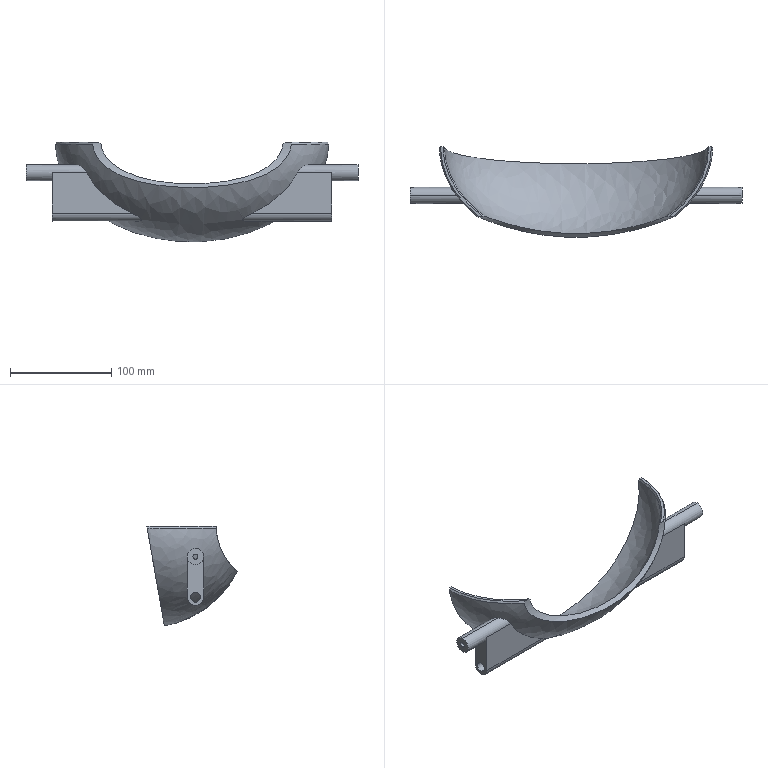Part | SolidWorks | features ICE 3, MirrorPattern 2, 3DProfileFeature 1, Attribute 1, Chamfer 1, Revolution 1 | 1 solid | 37 faces | box 328 x 89.443 x 98.481 mm | volume 199314 mm3 | cylinder 16 | plane 11 | spline 10 | commonest cylinder face diameters 16 x7 5 x4 10 x4 116.808 x1